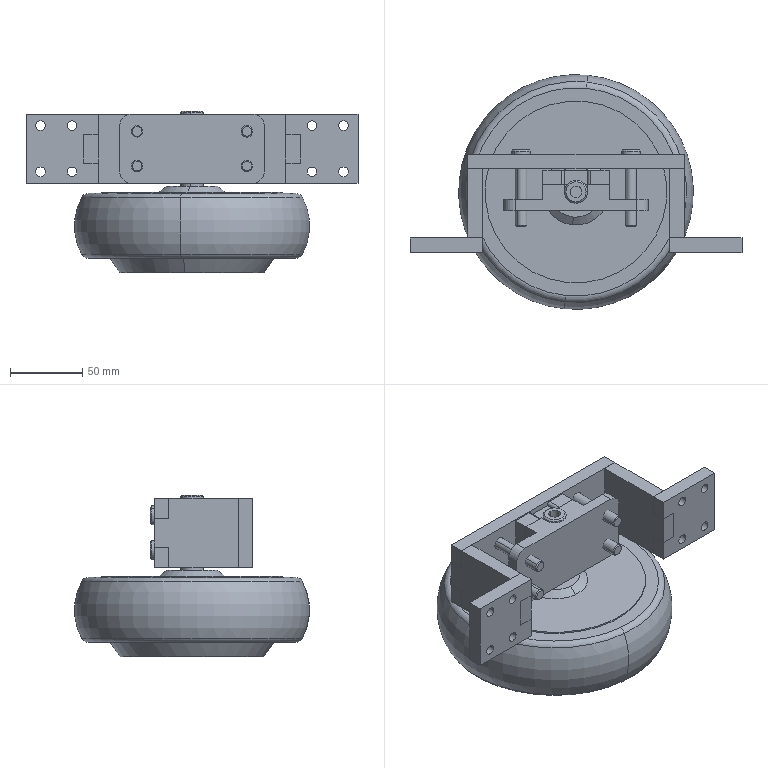Part | SolidWorks | 12 solids | 376 faces | box 230 x 163 x 112 mm | volume 1242773 mm3 | plane 177 | cylinder 115 | cone 70 | torus 14 | commonest cylinder face diameters 8 x18 6.6 x16 11 x16 15 x10 3.3 x8 4.5 x8